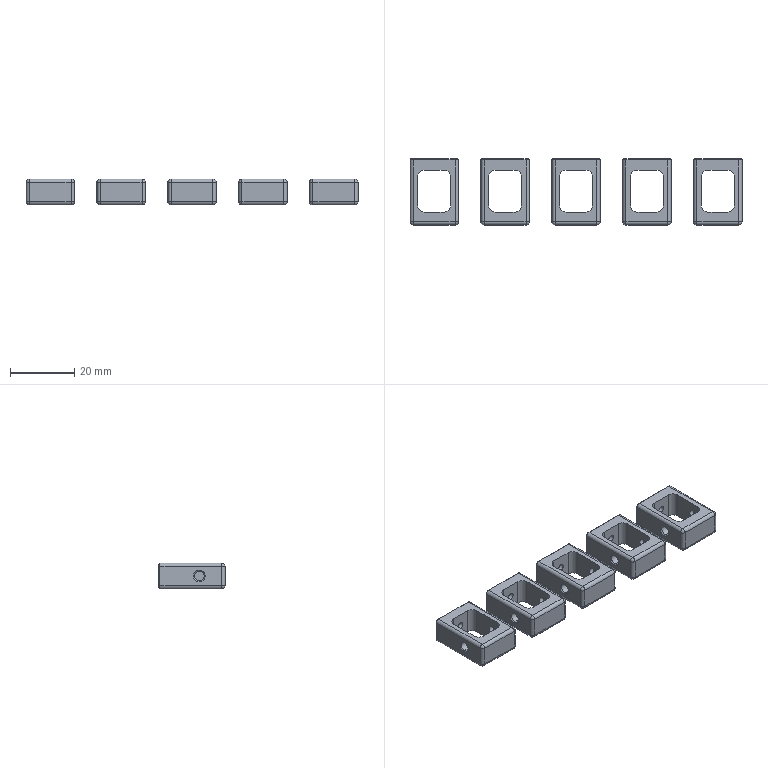Part | 5 solids | 215 faces | box 103 x 20.5 x 8 mm | volume 6792 mm3 | cylinder 90 | plane 75 | cone 30 | sphere 20 | commonest cylinder face diameters 2 x40 3 x20 4 x20 2.05 x10